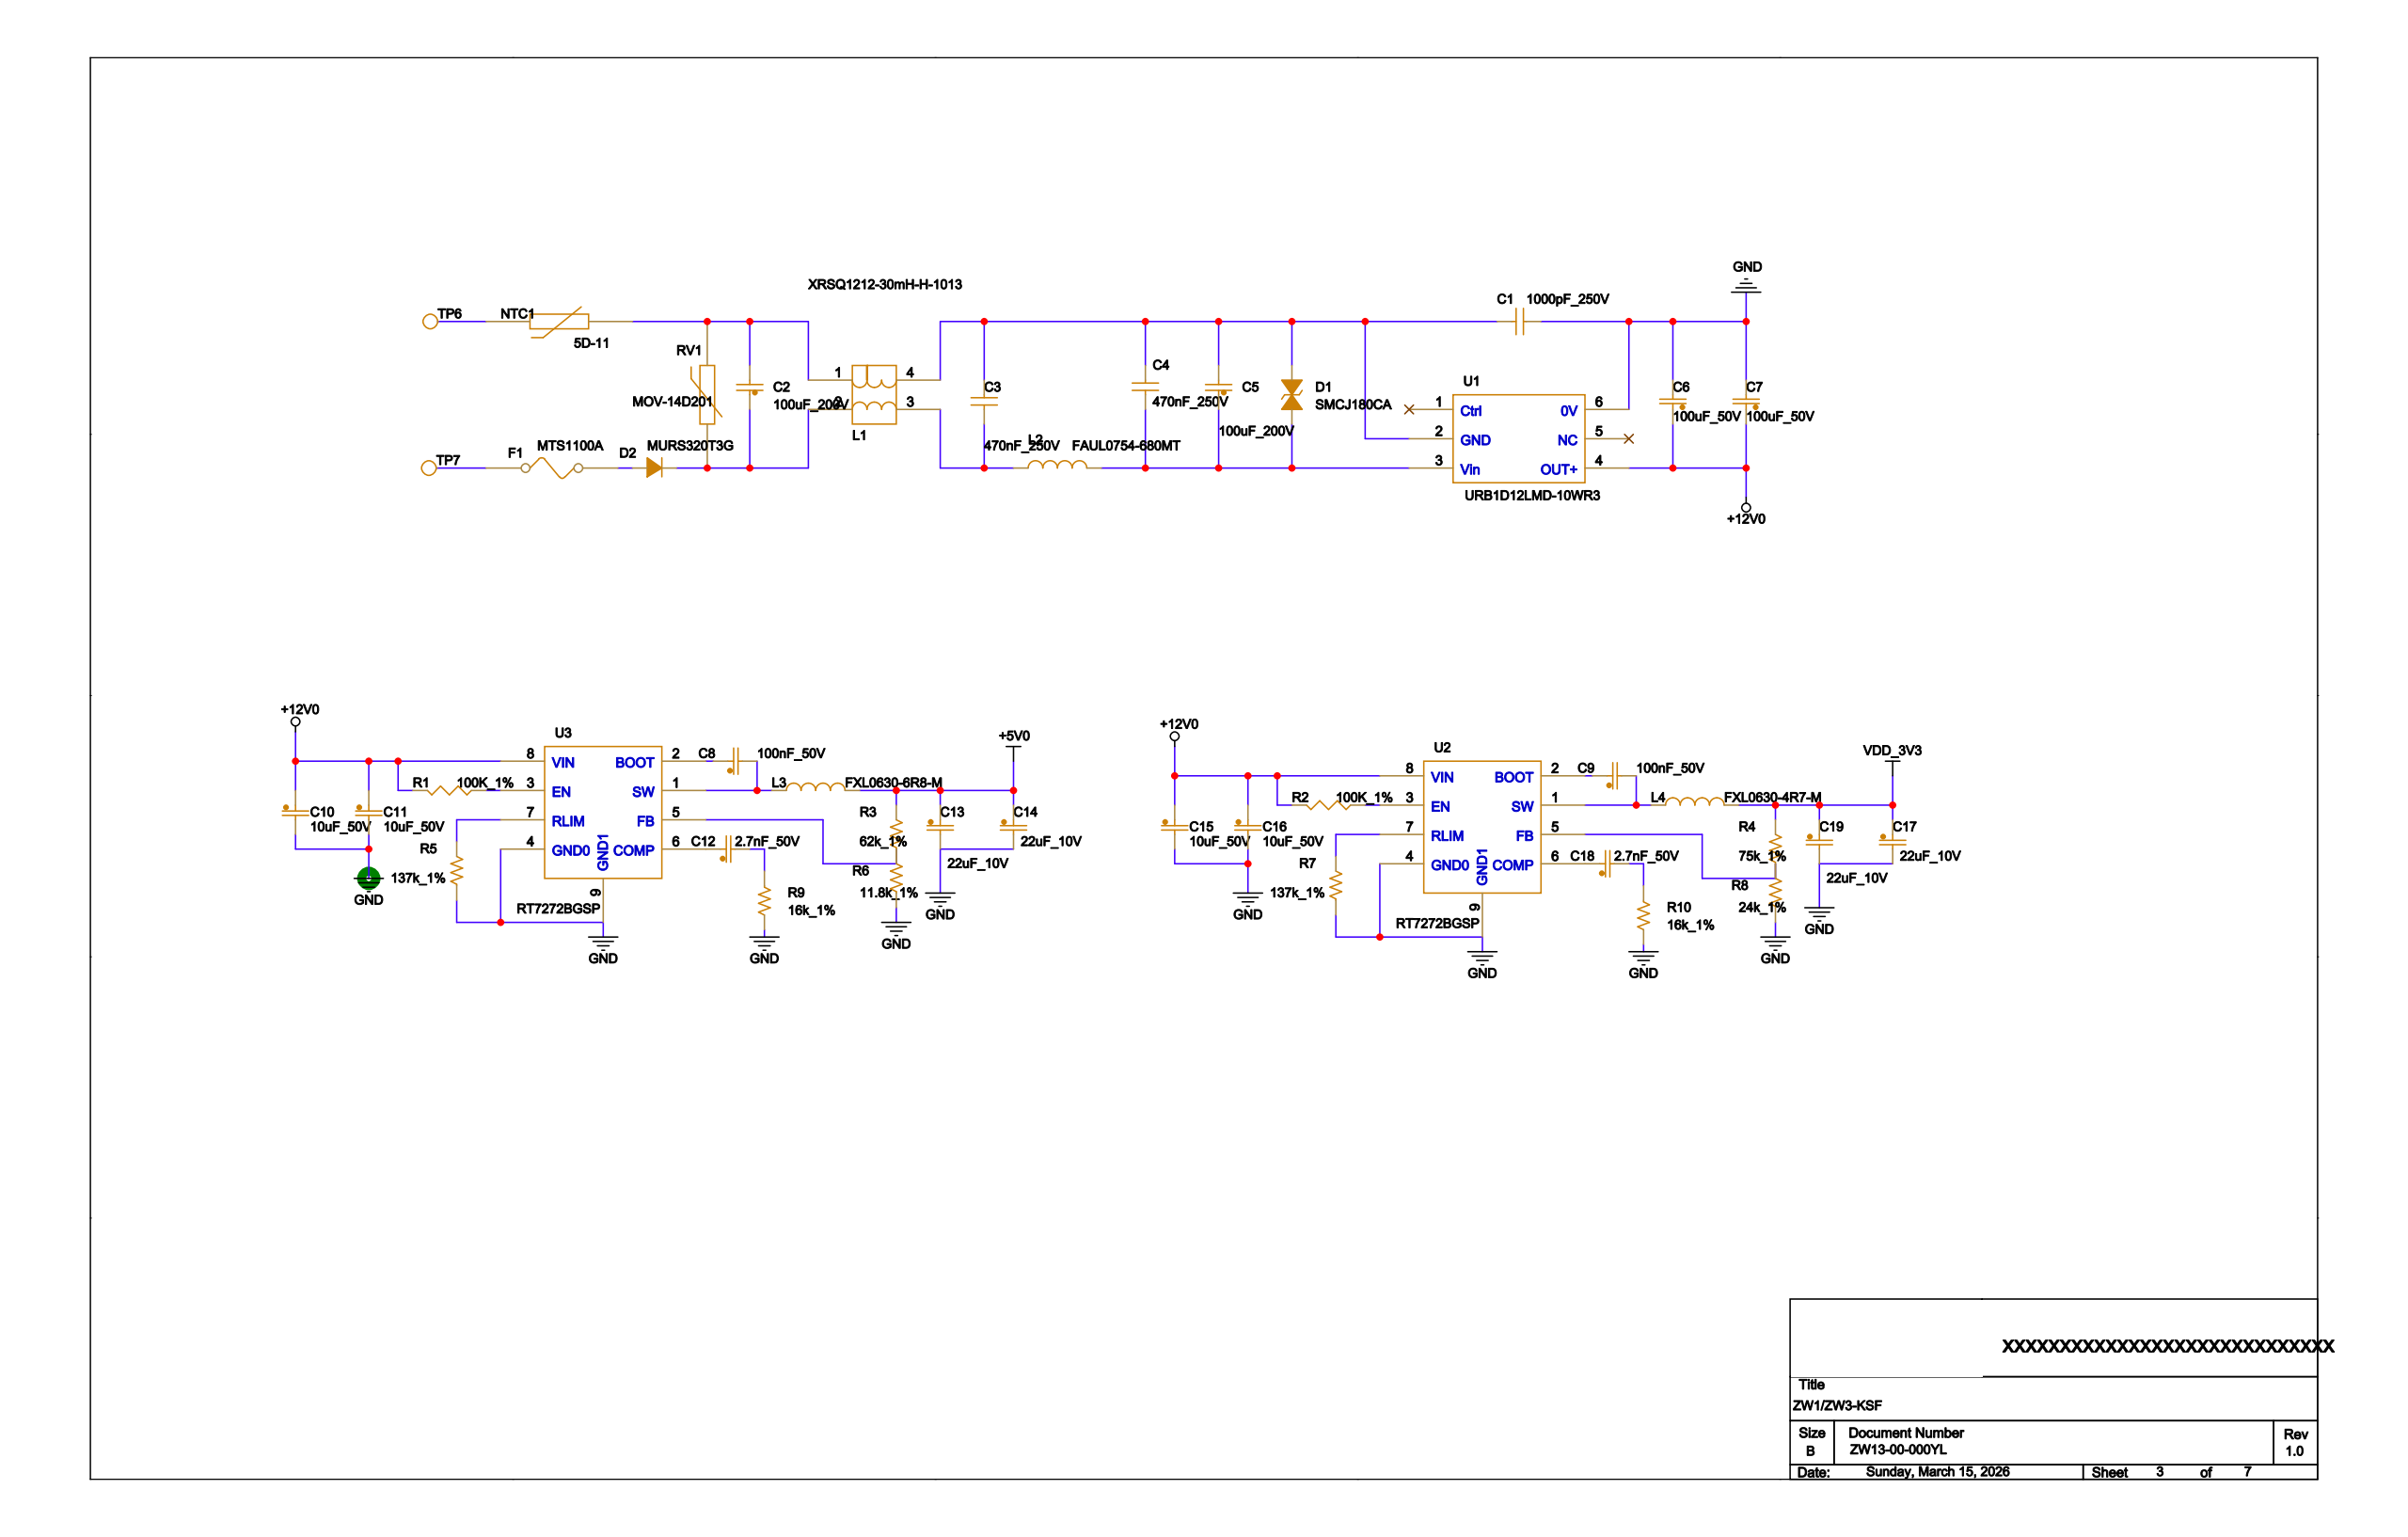Circuit board | Cadence Allegro | 260 parts | 211 nets | one sheet of the schematic
Parts on this sheet (reference | value | footprint):
C1 | CAP-TH_L10_0-W5_0-P10_00-D0_6
C2 | CAP-TH_BD16_0-P7_50-D0_8-FD
C3 | CAP-TH_L26_5-W10_0-P22_50-D1_4
C4 | CAP-TH_L26_5-W10_0-P22_50-D1_4
C5 | CAP-TH_BD16_0-P7_50-D0_8-FD
C6 | CAP-SMD_BD8_0-L8_3-W8_3-LS9_0-FD_H10_2
C7 | CAP-SMD_BD8_0-L8_3-W8_3-LS9_0-FD_H10_2
C8 | 0603-C
C9 | 0603-C
C10 | 1206-C
C11 | 1206-C
C12 | 0603-C
C13 | 0805-C
C14 | 0805-C
C15 | 1206-C
C16 | 1206-C
C17 | 0805-C
C18 | 0603-C
C19 | 0805-C
F1 | FUSE-TH_L8_4-W4_0-P5_08-D0_6
L1 | FL2D-30-103
L2 | IND-SMD_L7_9-W7_2
L3 | SMD_LDPC0530RCP
L4 | SMD_LDPC0530RCP
NTC1 | RES-TH_L12_5-W6_5-P7_50-D1_2-S6_3
R1 | R0603
R2 | R0603
R3 | R0603
R4 | R0603
R5 | R0603
R6 | R0603
R7 | R0603
R8 | R0603
R9 | R0603
R10 | R0603
RV1 | RES-TH_L16_5-W4_2-P7_50-D1_2-S1_90
TP6 | TP52_80
TP7 | TP52_80
U1 | PWRM-TH_5P-L50_8-W25_4-P5_08_URB1D24LMD-10WR3
U2 | SMD_DDA
U3 | SMD_DDA
Nets of these parts (net: part-pin ...):
GND: C1-1 C6-2 C7-2 C10-2 C11-2 C13-2 C14-2 C15-2 C16-2 C17-2 C19-2 R5-1 R6-1 R7-1 R8-1 R9-2 R10-2 U1-6 U2-4 U2-9 U3-4 U3-9
N17186669: C1-2 C3-1 C4-1 C5-2 L1-4 U1-2
+12V0: C6-1 C7-1 C10-1 C11-1 C15-1 C16-1 R1-2 R2-2 U1-4 U2-8 U3-8
VDD_3V3: C17-1 C19-1 L4-2 R4-2
N171871605: C12-1 U3-6
N17187304: C12-2 R9-1
N171876275: C18-1 U2-6
N17187771: C18-2 R10-1
+5V0: C13-1 C14-1 L3-2 R3-2
N17186783: C2-1 L1-2 RV1-1
N17186663: C2-2 L1-1 NTC1-1 RV1-2
N17186793: C4-2 C5-1 L2-2 U1-3
N17187188: C8-1 U3-2
N17187190: C8-2 L3-1 U3-1
N17187655: C9-1 U2-2
N17187657: C9-2 L4-1 U2-1
N17186785: C3-2 L1-3 L2-1
N17186836: F1-2
N17284215: F1-1 TP7-1
N17284201: NTC1-2 TP6-1
N17187212: R1-1 U3-3
N17187679: R2-1 U2-3
N17187250: R3-1 R6-2 U3-5
N17187717: R4-1 R8-2 U2-5
N17187246: R5-2 U3-7
N17187713: R7-2 U2-7